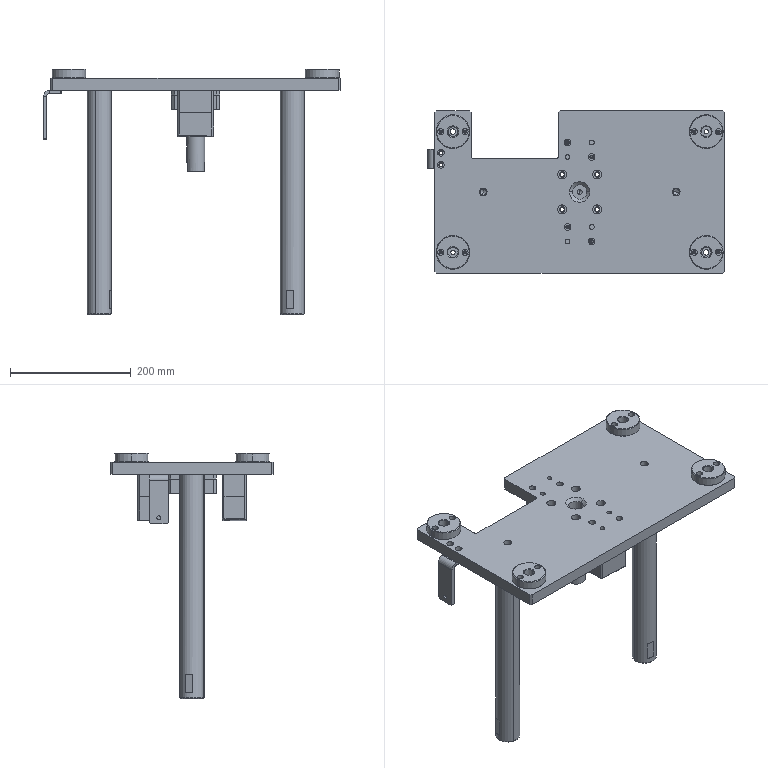Part | SolidWorks | 15 solids | 530 faces | box 492 x 270 x 407 mm | volume 3967388 mm3 | cylinder 238 | plane 174 | cone 114 | torus 4 | commonest cylinder face diameters 8 x32 5 x20 6.6 x20 9 x20 11 x20 10 x19